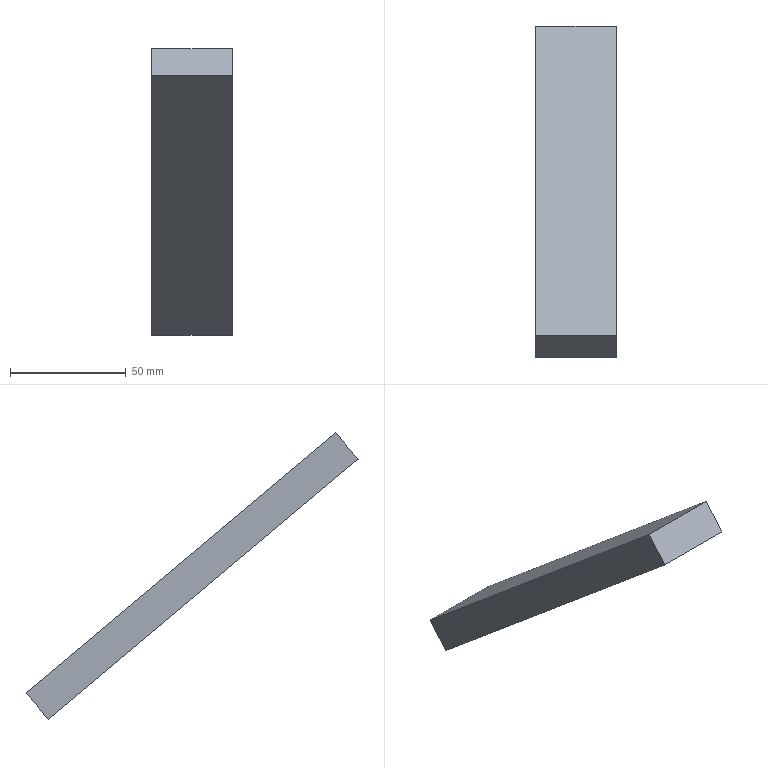Part | NX | features solid 2 | 1 solid | 6 faces | box 35 x 143.7 x 123.978 mm | volume 91875 mm3 | plane 6
STEP:
#1=CARTESIAN_POINT('',(245.,1029.809,-239.287));
#2=VERTEX_POINT('',#1);
#3=CARTESIAN_POINT('',(245.,1020.167,-250.778));
#4=VERTEX_POINT('',#3);
#5=CARTESIAN_POINT('',(245.,1029.809,-239.287));
#6=DIRECTION('',(0.,-0.6428,-0.766));
#7=VECTOR('',#6,1000.);
#8=LINE('',#5,#7);
#9=EDGE_CURVE('',#2,#4,#8,.T.);
#10=ORIENTED_EDGE('',*,*,#9,.T.);
#11=CARTESIAN_POINT('',(210.,1020.167,-250.778));
#12=VERTEX_POINT('',#11);
#13=CARTESIAN_POINT('',(210.,1020.167,-250.778));
#14=DIRECTION('',(1.,0.,0.));
#15=VECTOR('',#14,1000.);
#16=LINE('',#13,#15);
#17=EDGE_CURVE('',#12,#4,#16,.T.);
#18=ORIENTED_EDGE('',*,*,#17,.F.);
#19=CARTESIAN_POINT('',(210.,1029.809,-239.287));
#20=VERTEX_POINT('',#19);
#21=CARTESIAN_POINT('',(210.,1029.809,-239.287));
#22=DIRECTION('',(0.,-0.6428,-0.766));
#23=VECTOR('',#22,1000.);
#24=LINE('',#21,#23);
#25=EDGE_CURVE('',#20,#12,#24,.T.);
#26=ORIENTED_EDGE('',*,*,#25,.F.);
#27=CARTESIAN_POINT('',(210.,1029.809,-239.287));
#28=DIRECTION('',(1.,0.,0.));
#29=VECTOR('',#28,1000.);
#30=LINE('',#27,#29);
#31=EDGE_CURVE('',#20,#2,#30,.T.);
#32=ORIENTED_EDGE('',*,*,#31,.T.);
#33=EDGE_LOOP('',(#10,#18,#26,#32));
#34=FACE_BOUND('',#33,.T.);
#35=CARTESIAN_POINT('',(210.,1029.809,-239.287));
#36=DIRECTION('',(0.,0.766,-0.6428));
#37=DIRECTION('',(0.,-0.6428,-0.766));
#38=AXIS2_PLACEMENT_3D('',#35,#36,#37);
#39=PLANE('',#38);
#40=ADVANCED_FACE('',(#34),#39,.T.);
#41=CARTESIAN_POINT('',(245.,886.11,-138.29));
#42=VERTEX_POINT('',#41);
#43=CARTESIAN_POINT('',(210.,886.11,-138.29));
#44=VERTEX_POINT('',#43);
#45=CARTESIAN_POINT('',(210.,886.11,-138.29));
#46=DIRECTION('',(-1.,0.,0.));
#47=VECTOR('',#46,1000.);
#48=LINE('',#45,#47);
#49=EDGE_CURVE('',#42,#44,#48,.T.);
#50=ORIENTED_EDGE('',*,*,#49,.T.);
#51=CARTESIAN_POINT('',(210.,1020.167,-250.778));
#52=DIRECTION('',(0.,-0.766,0.6428));
#53=VECTOR('',#52,1000.);
#54=LINE('',#51,#53);
#55=EDGE_CURVE('',#12,#44,#54,.T.);
#56=ORIENTED_EDGE('',*,*,#55,.F.);
#57=ORIENTED_EDGE('',*,*,#17,.T.);
#58=CARTESIAN_POINT('',(245.,1020.167,-250.778));
#59=DIRECTION('',(0.,-0.766,0.6428));
#60=VECTOR('',#59,1000.);
#61=LINE('',#58,#60);
#62=EDGE_CURVE('',#4,#42,#61,.T.);
#63=ORIENTED_EDGE('',*,*,#62,.T.);
#64=EDGE_LOOP('',(#50,#56,#57,#63));
#65=FACE_BOUND('',#64,.T.);
#66=CARTESIAN_POINT('',(210.,1020.167,-250.778));
#67=DIRECTION('',(0.,-0.6428,-0.766));
#68=DIRECTION('',(0.,-0.766,0.6428));
#69=AXIS2_PLACEMENT_3D('',#66,#67,#68);
#70=PLANE('',#69);
#71=ADVANCED_FACE('',(#65),#70,.T.);
#72=CARTESIAN_POINT('',(245.,895.751,-126.799));
#73=VERTEX_POINT('',#72);
#74=CARTESIAN_POINT('',(245.,1029.809,-239.287));
#75=DIRECTION('',(0.,-0.766,0.6428));
#76=VECTOR('',#75,1000.);
#77=LINE('',#74,#76);
#78=EDGE_CURVE('',#2,#73,#77,.T.);
#79=ORIENTED_EDGE('',*,*,#78,.F.);
#80=ORIENTED_EDGE('',*,*,#31,.F.);
#81=CARTESIAN_POINT('',(210.,895.751,-126.799));
#82=VERTEX_POINT('',#81);
#83=CARTESIAN_POINT('',(210.,1029.809,-239.287));
#84=DIRECTION('',(0.,-0.766,0.6428));
#85=VECTOR('',#84,1000.);
#86=LINE('',#83,#85);
#87=EDGE_CURVE('',#20,#82,#86,.T.);
#88=ORIENTED_EDGE('',*,*,#87,.T.);
#89=CARTESIAN_POINT('',(210.,895.751,-126.799));
#90=DIRECTION('',(-1.,0.,0.));
#91=VECTOR('',#90,1000.);
#92=LINE('',#89,#91);
#93=EDGE_CURVE('',#73,#82,#92,.T.);
#94=ORIENTED_EDGE('',*,*,#93,.F.);
#95=EDGE_LOOP('',(#79,#80,#88,#94));
#96=FACE_BOUND('',#95,.T.);
#97=CARTESIAN_POINT('',(210.,1029.809,-239.287));
#98=DIRECTION('',(0.,-0.6428,-0.766));
#99=DIRECTION('',(0.,-0.766,0.6428));
#100=AXIS2_PLACEMENT_3D('',#97,#98,#99);
#101=PLANE('',#100);
#102=ADVANCED_FACE('',(#96),#101,.F.);
#103=ORIENTED_EDGE('',*,*,#87,.F.);
#104=ORIENTED_EDGE('',*,*,#25,.T.);
#105=ORIENTED_EDGE('',*,*,#55,.T.);
#106=CARTESIAN_POINT('',(210.,886.11,-138.29));
#107=DIRECTION('',(0.,-0.6428,-0.766));
#108=VECTOR('',#107,1000.);
#109=LINE('',#106,#108);
#110=EDGE_CURVE('',#82,#44,#109,.T.);
#111=ORIENTED_EDGE('',*,*,#110,.F.);
#112=EDGE_LOOP('',(#103,#104,#105,#111));
#113=FACE_BOUND('',#112,.T.);
#114=CARTESIAN_POINT('',(210.,1020.167,-250.778));
#115=DIRECTION('',(1.,0.,0.));
#116=DIRECTION('',(0.,-0.9397,0.342));
#117=AXIS2_PLACEMENT_3D('',#114,#115,#116);
#118=PLANE('',#117);
#119=ADVANCED_FACE('',(#113),#118,.F.);
#120=CARTESIAN_POINT('',(245.,886.11,-138.29));
#121=DIRECTION('',(0.,-0.6428,-0.766));
#122=VECTOR('',#121,1000.);
#123=LINE('',#120,#122);
#124=EDGE_CURVE('',#73,#42,#123,.T.);
#125=ORIENTED_EDGE('',*,*,#124,.T.);
#126=ORIENTED_EDGE('',*,*,#62,.F.);
#127=ORIENTED_EDGE('',*,*,#9,.F.);
#128=ORIENTED_EDGE('',*,*,#78,.T.);
#129=EDGE_LOOP('',(#125,#126,#127,#128));
#130=FACE_BOUND('',#129,.T.);
#131=CARTESIAN_POINT('',(245.,1020.167,-250.778));
#132=DIRECTION('',(1.,0.,0.));
#133=DIRECTION('',(0.,-0.9397,0.342));
#134=AXIS2_PLACEMENT_3D('',#131,#132,#133);
#135=PLANE('',#134);
#136=ADVANCED_FACE('',(#130),#135,.T.);
#137=ORIENTED_EDGE('',*,*,#110,.T.);
#138=ORIENTED_EDGE('',*,*,#49,.F.);
#139=ORIENTED_EDGE('',*,*,#124,.F.);
#140=ORIENTED_EDGE('',*,*,#93,.T.);
#141=EDGE_LOOP('',(#137,#138,#139,#140));
#142=FACE_BOUND('',#141,.T.);
#143=CARTESIAN_POINT('',(245.,960.673,-49.429));
#144=DIRECTION('',(0.,0.766,-0.6428));
#145=DIRECTION('',(0.,-0.6428,-0.766));
#146=AXIS2_PLACEMENT_3D('',#143,#144,#145);
#147=PLANE('',#146);
#148=ADVANCED_FACE('',(#142),#147,.F.);
#149=CLOSED_SHELL('',(#40,#71,#102,#119,#136,#148));
#150=MANIFOLD_SOLID_BREP('',#149);
#151=(LENGTH_UNIT()NAMED_UNIT(*)SI_UNIT(.MILLI.,.METRE.));
#152=UNCERTAINTY_MEASURE_WITH_UNIT(LENGTH_MEASURE(0.00001),#151,'','');
#153=(NAMED_UNIT(*)PLANE_ANGLE_UNIT()SI_UNIT($,.RADIAN.));
#154=(NAMED_UNIT(*)SI_UNIT($,.STERADIAN.)SOLID_ANGLE_UNIT());
#155=(GEOMETRIC_REPRESENTATION_CONTEXT(3)GLOBAL_UNCERTAINTY_ASSIGNED_CONTEXT((#152))GLOBAL_UNIT_ASSIGNED_CONTEXT((#151,#153,#154))REPRESENTATION_CONTEXT('',''));
#156=ADVANCED_BREP_SHAPE_REPRESENTATION('',(#150),#155);